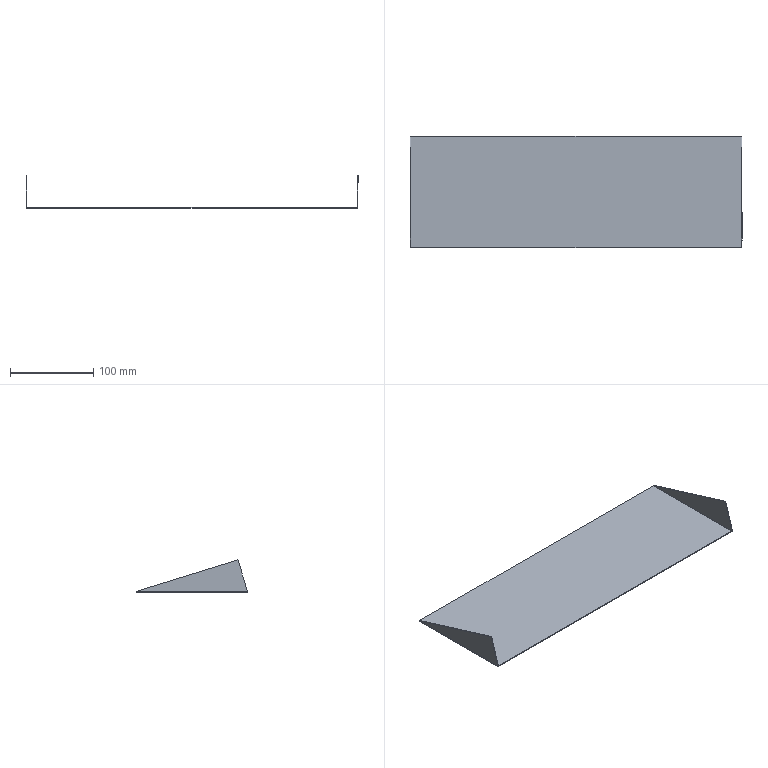Part | SolidWorks | features EdgeFlange 1, FlatPattern 1, MirrorPattern 1, SMBaseFlange 1, SheetMetal 1 | 1 solid | 20 faces | box 399.001 x 133.5 x 38.5 mm | volume 58192 mm3 | plane 12 | spline 4 | cylinder 4 | commonest cylinder face diameters 0.4 x2 2.4 x2
STEP:
#1=CARTESIAN_POINT('',(198.3,66.75,-1.));
#2=VERTEX_POINT('',#1);
#3=CARTESIAN_POINT('',(198.3,-66.75,-1.));
#4=VERTEX_POINT('',#3);
#5=CARTESIAN_POINT('',(198.3,66.75,-1.));
#6=DIRECTION('',(0.,-1.,0.));
#7=VECTOR('',#6,1000.);
#8=LINE('',#5,#7);
#9=EDGE_CURVE('',#2,#4,#8,.T.);
#10=ORIENTED_EDGE('',*,*,#9,.T.);
#11=CARTESIAN_POINT('',(-198.3,-66.75,-1.));
#12=VERTEX_POINT('',#11);
#13=CARTESIAN_POINT('',(-199.5,-66.75,-1.));
#14=DIRECTION('',(1.,0.,0.));
#15=VECTOR('',#14,1000.);
#16=LINE('',#13,#15);
#17=EDGE_CURVE('',#12,#4,#16,.T.);
#18=ORIENTED_EDGE('',*,*,#17,.F.);
#19=CARTESIAN_POINT('',(-198.3,66.75,-1.));
#20=VERTEX_POINT('',#19);
#21=CARTESIAN_POINT('',(-198.3,-66.75,-1.));
#22=DIRECTION('',(0.,1.,0.));
#23=VECTOR('',#22,1000.);
#24=LINE('',#21,#23);
#25=EDGE_CURVE('',#12,#20,#24,.T.);
#26=ORIENTED_EDGE('',*,*,#25,.T.);
#27=CARTESIAN_POINT('',(-199.5,66.75,-1.));
#28=DIRECTION('',(-1.,0.,0.));
#29=VECTOR('',#28,1000.);
#30=LINE('',#27,#29);
#31=EDGE_CURVE('',#2,#20,#30,.T.);
#32=ORIENTED_EDGE('',*,*,#31,.F.);
#33=EDGE_LOOP('',(#10,#18,#26,#32));
#34=FACE_OUTER_BOUND('',#33,.T.);
#35=CARTESIAN_POINT('',(0.,0.,-1.));
#36=DIRECTION('',(0.,0.,1.));
#37=DIRECTION('',(1.,0.,0.));
#38=AXIS2_PLACEMENT_3D('',#35,#36,#37);
#39=PLANE('',#38);
#40=ADVANCED_FACE('',(#34),#39,.F.);
#41=CARTESIAN_POINT('',(-198.3,-66.75,0.));
#42=VERTEX_POINT('',#41);
#43=CARTESIAN_POINT('',(198.3,-66.75,0.));
#44=VERTEX_POINT('',#43);
#45=CARTESIAN_POINT('',(-199.5,-66.75,0.));
#46=DIRECTION('',(1.,0.,0.));
#47=VECTOR('',#46,1000.);
#48=LINE('',#45,#47);
#49=EDGE_CURVE('',#42,#44,#48,.T.);
#50=ORIENTED_EDGE('',*,*,#49,.T.);
#51=CARTESIAN_POINT('',(198.3,66.75,0.));
#52=VERTEX_POINT('',#51);
#53=CARTESIAN_POINT('',(198.3,66.75,0.));
#54=DIRECTION('',(0.,-1.,0.));
#55=VECTOR('',#54,1000.);
#56=LINE('',#53,#55);
#57=EDGE_CURVE('',#52,#44,#56,.T.);
#58=ORIENTED_EDGE('',*,*,#57,.F.);
#59=CARTESIAN_POINT('',(-198.3,66.75,0.));
#60=VERTEX_POINT('',#59);
#61=CARTESIAN_POINT('',(-199.5,66.75,0.));
#62=DIRECTION('',(-1.,0.,0.));
#63=VECTOR('',#62,1000.);
#64=LINE('',#61,#63);
#65=EDGE_CURVE('',#52,#60,#64,.T.);
#66=ORIENTED_EDGE('',*,*,#65,.T.);
#67=CARTESIAN_POINT('',(-198.3,-66.75,0.));
#68=DIRECTION('',(0.,1.,0.));
#69=VECTOR('',#68,1000.);
#70=LINE('',#67,#69);
#71=EDGE_CURVE('',#42,#60,#70,.T.);
#72=ORIENTED_EDGE('',*,*,#71,.F.);
#73=EDGE_LOOP('',(#50,#58,#66,#72));
#74=FACE_OUTER_BOUND('',#73,.T.);
#75=CARTESIAN_POINT('',(0.,0.,0.));
#76=DIRECTION('',(0.,0.,1.));
#77=DIRECTION('',(1.,0.,0.));
#78=AXIS2_PLACEMENT_3D('',#75,#76,#77);
#79=PLANE('',#78);
#80=ADVANCED_FACE('',(#74),#79,.T.);
#81=ORIENTED_EDGE('',*,*,#65,.F.);
#82=CARTESIAN_POINT('',(198.3,66.75,0.));
#83=DIRECTION('',(0.,0.,-1.));
#84=VECTOR('',#83,1000.);
#85=LINE('',#82,#84);
#86=EDGE_CURVE('',#52,#2,#85,.T.);
#87=ORIENTED_EDGE('',*,*,#86,.T.);
#88=ORIENTED_EDGE('',*,*,#31,.T.);
#89=CARTESIAN_POINT('',(-198.3,66.75,0.));
#90=DIRECTION('',(0.,0.,-1.));
#91=VECTOR('',#90,1000.);
#92=LINE('',#89,#91);
#93=EDGE_CURVE('',#60,#20,#92,.T.);
#94=ORIENTED_EDGE('',*,*,#93,.F.);
#95=EDGE_LOOP('',(#81,#87,#88,#94));
#96=FACE_OUTER_BOUND('',#95,.T.);
#97=CARTESIAN_POINT('',(-199.5,66.75,-1.));
#98=DIRECTION('',(0.,1.,0.));
#99=DIRECTION('',(0.,0.,1.));
#100=AXIS2_PLACEMENT_3D('',#97,#98,#99);
#101=PLANE('',#100);
#102=ADVANCED_FACE('',(#96),#101,.T.);
#103=CARTESIAN_POINT('',(198.3,-66.75,0.));
#104=DIRECTION('',(0.,0.,-1.));
#105=VECTOR('',#104,1000.);
#106=LINE('',#103,#105);
#107=EDGE_CURVE('',#44,#4,#106,.T.);
#108=ORIENTED_EDGE('',*,*,#107,.F.);
#109=ORIENTED_EDGE('',*,*,#49,.F.);
#110=CARTESIAN_POINT('',(-198.3,-66.75,0.));
#111=DIRECTION('',(0.,0.,-1.));
#112=VECTOR('',#111,1000.);
#113=LINE('',#110,#112);
#114=EDGE_CURVE('',#42,#12,#113,.T.);
#115=ORIENTED_EDGE('',*,*,#114,.T.);
#116=ORIENTED_EDGE('',*,*,#17,.T.);
#117=EDGE_LOOP('',(#108,#109,#115,#116));
#118=FACE_OUTER_BOUND('',#117,.T.);
#119=CARTESIAN_POINT('',(-199.5,-66.75,-1.));
#120=DIRECTION('',(0.,-1.,0.));
#121=DIRECTION('',(0.,0.,-1.));
#122=AXIS2_PLACEMENT_3D('',#119,#120,#121);
#123=PLANE('',#122);
#124=ADVANCED_FACE('',(#118),#123,.T.);
#125=CARTESIAN_POINT('',(-198.5,66.099,0.2));
#126=VERTEX_POINT('',#125);
#127=CARTESIAN_POINT('',(-199.5,66.099,0.2));
#128=VERTEX_POINT('',#127);
#129=CARTESIAN_POINT('',(-199.5,66.099,0.2));
#130=DIRECTION('',(-1.,0.,0.));
#131=VECTOR('',#130,1000.);
#132=LINE('',#129,#131);
#133=EDGE_CURVE('',#126,#128,#132,.T.);
#134=ORIENTED_EDGE('',*,*,#133,.F.);
#135=CARTESIAN_POINT('',(-198.3,66.75,0.));
#136=CARTESIAN_POINT('',(-198.352,66.642,0.));
#137=CARTESIAN_POINT('',(-198.404,66.533,0.02155));
#138=CARTESIAN_POINT('',(-198.478,66.316,0.0956));
#139=CARTESIAN_POINT('',(-198.5,66.208,0.1476));
#140=CARTESIAN_POINT('',(-198.5,66.099,0.2));
#141=B_SPLINE_CURVE_WITH_KNOTS('',3,(#135,#136,#137,#138,#139,#140),.UNSPECIFIED.,.F.,.F.,(4,2,4),(0.,0.5,1.),.UNSPECIFIED.);
#142=EDGE_CURVE('',#60,#126,#141,.T.);
#143=ORIENTED_EDGE('',*,*,#142,.F.);
#144=ORIENTED_EDGE('',*,*,#93,.T.);
#145=CARTESIAN_POINT('',(-198.3,66.75,-1.));
#146=CARTESIAN_POINT('',(-198.459,66.695,-1.));
#147=CARTESIAN_POINT('',(-198.612,66.642,-0.9696));
#148=CARTESIAN_POINT('',(-198.904,66.533,-0.8489));
#149=CARTESIAN_POINT('',(-199.036,66.48,-0.761));
#150=CARTESIAN_POINT('',(-199.26,66.371,-0.5375));
#151=CARTESIAN_POINT('',(-199.348,66.317,-0.4053));
#152=CARTESIAN_POINT('',(-199.469,66.208,-0.1145));
#153=CARTESIAN_POINT('',(-199.5,66.154,0.04138));
#154=CARTESIAN_POINT('',(-199.5,66.099,0.2));
#155=B_SPLINE_CURVE_WITH_KNOTS('',3,(#145,#146,#147,#148,#149,#150,#151,#152,#153,#154),.UNSPECIFIED.,.F.,.F.,(4,2,2,2,4),(0.,0.0004941,0.0009882,0.001482,0.001976),.UNSPECIFIED.);
#156=EDGE_CURVE('',#20,#128,#155,.T.);
#157=ORIENTED_EDGE('',*,*,#156,.T.);
#158=EDGE_LOOP('',(#134,#143,#144,#157));
#159=FACE_OUTER_BOUND('',#158,.T.);
#160=CARTESIAN_POINT('',(-198.3,66.75,-1.01));
#161=CARTESIAN_POINT('',(-198.458,66.696,-1.01));
#162=CARTESIAN_POINT('',(-198.617,66.642,-0.9785));
#163=CARTESIAN_POINT('',(-198.909,66.533,-0.8573));
#164=CARTESIAN_POINT('',(-199.044,66.479,-0.7676));
#165=CARTESIAN_POINT('',(-199.268,66.371,-0.5436));
#166=CARTESIAN_POINT('',(-199.357,66.316,-0.4094));
#167=CARTESIAN_POINT('',(-199.479,66.208,-0.1167));
#168=CARTESIAN_POINT('',(-199.51,66.154,0.04159));
#169=CARTESIAN_POINT('',(-199.51,66.099,0.2));
#170=CARTESIAN_POINT('',(-198.3,66.75,-1.));
#171=CARTESIAN_POINT('',(-198.457,66.696,-1.));
#172=CARTESIAN_POINT('',(-198.614,66.642,-0.9688));
#173=CARTESIAN_POINT('',(-198.904,66.533,-0.8485));
#174=CARTESIAN_POINT('',(-199.037,66.479,-0.7596));
#175=CARTESIAN_POINT('',(-199.26,66.371,-0.5375));
#176=CARTESIAN_POINT('',(-199.349,66.316,-0.4043));
#177=CARTESIAN_POINT('',(-199.469,66.208,-0.1141));
#178=CARTESIAN_POINT('',(-199.5,66.154,0.0429));
#179=CARTESIAN_POINT('',(-199.5,66.099,0.2));
#180=CARTESIAN_POINT('',(-198.3,66.75,0.));
#181=CARTESIAN_POINT('',(-198.326,66.696,0.));
#182=CARTESIAN_POINT('',(-198.352,66.642,0.005205));
#183=CARTESIAN_POINT('',(-198.401,66.533,0.02524));
#184=CARTESIAN_POINT('',(-198.423,66.479,0.04007));
#185=CARTESIAN_POINT('',(-198.46,66.371,0.07709));
#186=CARTESIAN_POINT('',(-198.475,66.316,0.09928));
#187=CARTESIAN_POINT('',(-198.495,66.208,0.1477));
#188=CARTESIAN_POINT('',(-198.5,66.154,0.1738));
#189=CARTESIAN_POINT('',(-198.5,66.099,0.2));
#190=B_SPLINE_SURFACE_WITH_KNOTS('',1,3,((#160,#161,#162,#163,#164,#165,#166,#167,#168,#169),(#170,#171,#172,#173,#174,#175,#176,#177,#178,#179),(#180,#181,#182,#183,#184,#185,#186,#187,#188,#189)),.UNSPECIFIED.,.F.,.F.,.F.,(2,1,2),(4,2,2,2,4),(-0.01,0.,1.),(0.,0.25,0.5,0.75,1.),.UNSPECIFIED.);
#191=ADVANCED_FACE('',(#159),#190,.F.);
#192=CARTESIAN_POINT('',(-198.5,-66.689,0.2));
#193=VERTEX_POINT('',#192);
#194=CARTESIAN_POINT('',(-198.5,-66.689,0.2));
#195=CARTESIAN_POINT('',(-198.5,-66.699,0.1476));
#196=CARTESIAN_POINT('',(-198.478,-66.709,0.0956));
#197=CARTESIAN_POINT('',(-198.404,-66.73,0.02155));
#198=CARTESIAN_POINT('',(-198.352,-66.74,0.));
#199=CARTESIAN_POINT('',(-198.3,-66.75,0.));
#200=B_SPLINE_CURVE_WITH_KNOTS('',3,(#194,#195,#196,#197,#198,#199),.UNSPECIFIED.,.F.,.F.,(4,2,4),(0.,0.5,1.),.UNSPECIFIED.);
#201=EDGE_CURVE('',#193,#42,#200,.T.);
#202=ORIENTED_EDGE('',*,*,#201,.F.);
#203=CARTESIAN_POINT('',(-199.5,-66.689,0.2));
#204=VERTEX_POINT('',#203);
#205=CARTESIAN_POINT('',(-198.5,-66.689,0.2));
#206=DIRECTION('',(-1.,0.,0.));
#207=VECTOR('',#206,1000.);
#208=LINE('',#205,#207);
#209=EDGE_CURVE('',#193,#204,#208,.T.);
#210=ORIENTED_EDGE('',*,*,#209,.T.);
#211=CARTESIAN_POINT('',(-199.5,-66.689,0.2));
#212=CARTESIAN_POINT('',(-199.5,-66.694,0.04292));
#213=CARTESIAN_POINT('',(-199.469,-66.699,-0.1141));
#214=CARTESIAN_POINT('',(-199.349,-66.709,-0.4043));
#215=CARTESIAN_POINT('',(-199.26,-66.714,-0.5375));
#216=CARTESIAN_POINT('',(-199.037,-66.724,-0.7596));
#217=CARTESIAN_POINT('',(-198.904,-66.73,-0.8485));
#218=CARTESIAN_POINT('',(-198.614,-66.74,-0.9688));
#219=CARTESIAN_POINT('',(-198.457,-66.745,-1.));
#220=CARTESIAN_POINT('',(-198.3,-66.75,-1.));
#221=B_SPLINE_CURVE_WITH_KNOTS('',3,(#211,#212,#213,#214,#215,#216,#217,#218,#219,#220),.UNSPECIFIED.,.F.,.F.,(4,2,2,2,4),(0.,0.25,0.5,0.75,1.),.UNSPECIFIED.);
#222=EDGE_CURVE('',#204,#12,#221,.T.);
#223=ORIENTED_EDGE('',*,*,#222,.T.);
#224=ORIENTED_EDGE('',*,*,#114,.F.);
#225=EDGE_LOOP('',(#202,#210,#223,#224));
#226=FACE_OUTER_BOUND('',#225,.T.);
#227=CARTESIAN_POINT('',(-199.51,-66.689,0.2));
#228=CARTESIAN_POINT('',(-199.51,-66.694,0.04158));
#229=CARTESIAN_POINT('',(-199.479,-66.699,-0.1167));
#230=CARTESIAN_POINT('',(-199.357,-66.709,-0.4094));
#231=CARTESIAN_POINT('',(-199.268,-66.714,-0.5436));
#232=CARTESIAN_POINT('',(-199.044,-66.724,-0.7676));
#233=CARTESIAN_POINT('',(-198.909,-66.73,-0.8573));
#234=CARTESIAN_POINT('',(-198.617,-66.74,-0.9785));
#235=CARTESIAN_POINT('',(-198.458,-66.745,-1.01));
#236=CARTESIAN_POINT('',(-198.3,-66.75,-1.01));
#237=CARTESIAN_POINT('',(-199.5,-66.689,0.2));
#238=CARTESIAN_POINT('',(-199.5,-66.694,0.04289));
#239=CARTESIAN_POINT('',(-199.469,-66.699,-0.1141));
#240=CARTESIAN_POINT('',(-199.349,-66.709,-0.4043));
#241=CARTESIAN_POINT('',(-199.26,-66.714,-0.5375));
#242=CARTESIAN_POINT('',(-199.037,-66.724,-0.7596));
#243=CARTESIAN_POINT('',(-198.904,-66.73,-0.8485));
#244=CARTESIAN_POINT('',(-198.614,-66.74,-0.9688));
#245=CARTESIAN_POINT('',(-198.457,-66.745,-1.));
#246=CARTESIAN_POINT('',(-198.3,-66.75,-1.));
#247=CARTESIAN_POINT('',(-198.5,-66.689,0.2));
#248=CARTESIAN_POINT('',(-198.5,-66.694,0.1738));
#249=CARTESIAN_POINT('',(-198.495,-66.699,0.1477));
#250=CARTESIAN_POINT('',(-198.475,-66.709,0.09928));
#251=CARTESIAN_POINT('',(-198.46,-66.714,0.07709));
#252=CARTESIAN_POINT('',(-198.423,-66.724,0.04007));
#253=CARTESIAN_POINT('',(-198.401,-66.73,0.02524));
#254=CARTESIAN_POINT('',(-198.352,-66.74,0.005205));
#255=CARTESIAN_POINT('',(-198.326,-66.745,0.));
#256=CARTESIAN_POINT('',(-198.3,-66.75,0.));
#257=CARTESIAN_POINT('',(-198.49,-66.689,0.2));
#258=CARTESIAN_POINT('',(-198.49,-66.694,0.1751));
#259=CARTESIAN_POINT('',(-198.485,-66.699,0.1503));
#260=CARTESIAN_POINT('',(-198.466,-66.709,0.1044));
#261=CARTESIAN_POINT('',(-198.452,-66.714,0.0833));
#262=CARTESIAN_POINT('',(-198.417,-66.724,0.04814));
#263=CARTESIAN_POINT('',(-198.396,-66.73,0.03407));
#264=CARTESIAN_POINT('',(-198.35,-66.74,0.01504));
#265=CARTESIAN_POINT('',(-198.325,-66.745,0.0101));
#266=CARTESIAN_POINT('',(-198.3,-66.75,0.0101));
#267=B_SPLINE_SURFACE_WITH_KNOTS('',1,3,((#227,#228,#229,#230,#231,#232,#233,#234,#235,#236),(#237,#238,#239,#240,#241,#242,#243,#244,#245,#246),(#247,#248,#249,#250,#251,#252,#253,#254,#255,#256),(#257,#258,#259,#260,#261,#262,#263,#264,#265,#266)),.UNSPECIFIED.,.F.,.F.,.F.,(2,1,1,2),(4,2,2,2,4),(-0.01,0.,1.,1.01),(0.,0.25,0.5,0.75,1.),.UNSPECIFIED.);
#268=ADVANCED_FACE('',(#226),#267,.F.);
#269=ORIENTED_EDGE('',*,*,#25,.F.);
#270=ORIENTED_EDGE('',*,*,#222,.F.);
#271=CARTESIAN_POINT('',(-199.5,66.099,0.2));
#272=DIRECTION('',(0.,1.,0.));
#273=VECTOR('',#272,1000.);
#274=LINE('',#271,#273);
#275=EDGE_CURVE('',#204,#128,#274,.T.);
#276=ORIENTED_EDGE('',*,*,#275,.T.);
#277=ORIENTED_EDGE('',*,*,#156,.F.);
#278=EDGE_LOOP('',(#269,#270,#276,#277));
#279=FACE_OUTER_BOUND('',#278,.T.);
#280=CARTESIAN_POINT('',(-198.3,-66.75,0.2));
#281=DIRECTION('',(0.,-1.,0.));
#282=DIRECTION('',(-1.,0.,0.));
#283=AXIS2_PLACEMENT_3D('',#280,#281,#282);
#284=CYLINDRICAL_SURFACE('',#283,1.2);
#285=ADVANCED_FACE('',(#279),#284,.T.);
#286=ORIENTED_EDGE('',*,*,#71,.T.);
#287=ORIENTED_EDGE('',*,*,#142,.T.);
#288=CARTESIAN_POINT('',(-198.5,66.099,0.2));
#289=DIRECTION('',(0.,-1.,0.));
#290=VECTOR('',#289,1000.);
#291=LINE('',#288,#290);
#292=EDGE_CURVE('',#126,#193,#291,.T.);
#293=ORIENTED_EDGE('',*,*,#292,.T.);
#294=ORIENTED_EDGE('',*,*,#201,.T.);
#295=EDGE_LOOP('',(#286,#287,#293,#294));
#296=FACE_OUTER_BOUND('',#295,.T.);
#297=CARTESIAN_POINT('',(-198.3,-66.75,0.2));
#298=DIRECTION('',(0.,-1.,0.));
#299=DIRECTION('',(-1.,0.,0.));
#300=AXIS2_PLACEMENT_3D('',#297,#298,#299);
#301=CYLINDRICAL_SURFACE('',#300,0.2);
#302=ADVANCED_FACE('',(#296),#301,.F.);
#303=ORIENTED_EDGE('',*,*,#133,.T.);
#304=CARTESIAN_POINT('',(-199.5,-55.221,37.5));
#305=VERTEX_POINT('',#304);
#306=CARTESIAN_POINT('',(-199.5,5.765,18.75));
#307=DIRECTION('',(0.,0.9558,-0.2939));
#308=VECTOR('',#307,1000.);
#309=LINE('',#306,#308);
#310=EDGE_CURVE('',#305,#128,#309,.T.);
#311=ORIENTED_EDGE('',*,*,#310,.F.);
#312=CARTESIAN_POINT('',(-198.5,-55.221,37.5));
#313=VERTEX_POINT('',#312);
#314=CARTESIAN_POINT('',(-199.5,-55.221,37.5));
#315=DIRECTION('',(1.,0.,0.));
#316=VECTOR('',#315,1000.);
#317=LINE('',#314,#316);
#318=EDGE_CURVE('',#305,#313,#317,.T.);
#319=ORIENTED_EDGE('',*,*,#318,.T.);
#320=CARTESIAN_POINT('',(-198.5,-55.221,37.5));
#321=DIRECTION('',(0.,0.9558,-0.2939));
#322=VECTOR('',#321,1000.);
#323=LINE('',#320,#322);
#324=EDGE_CURVE('',#313,#126,#323,.T.);
#325=ORIENTED_EDGE('',*,*,#324,.T.);
#326=EDGE_LOOP('',(#303,#311,#319,#325));
#327=FACE_OUTER_BOUND('',#326,.T.);
#328=CARTESIAN_POINT('',(-199.5,-55.221,37.5));
#329=DIRECTION('',(0.,-0.2939,-0.9558));
#330=DIRECTION('',(0.,0.9558,-0.2939));
#331=AXIS2_PLACEMENT_3D('',#328,#329,#330);
#332=PLANE('',#331);
#333=ADVANCED_FACE('',(#327),#332,.F.);
#334=ORIENTED_EDGE('',*,*,#209,.F.);
#335=CARTESIAN_POINT('',(-198.5,-66.75,0.));
#336=DIRECTION('',(0.,0.2939,0.9558));
#337=VECTOR('',#336,1000.);
#338=LINE('',#335,#337);
#339=EDGE_CURVE('',#193,#313,#338,.T.);
#340=ORIENTED_EDGE('',*,*,#339,.T.);
#341=ORIENTED_EDGE('',*,*,#318,.F.);
#342=CARTESIAN_POINT('',(-199.5,-60.985,18.75));
#343=DIRECTION('',(0.,0.2939,0.9558));
#344=VECTOR('',#343,1000.);
#345=LINE('',#342,#344);
#346=EDGE_CURVE('',#204,#305,#345,.T.);
#347=ORIENTED_EDGE('',*,*,#346,.F.);
#348=EDGE_LOOP('',(#334,#340,#341,#347));
#349=FACE_OUTER_BOUND('',#348,.T.);
#350=CARTESIAN_POINT('',(-199.5,-66.75,0.));
#351=DIRECTION('',(0.,0.9558,-0.2939));
#352=DIRECTION('',(0.,0.2939,0.9558));
#353=AXIS2_PLACEMENT_3D('',#350,#351,#352);
#354=PLANE('',#353);
#355=ADVANCED_FACE('',(#349),#354,.F.);
#356=ORIENTED_EDGE('',*,*,#275,.F.);
#357=ORIENTED_EDGE('',*,*,#346,.T.);
#358=ORIENTED_EDGE('',*,*,#310,.T.);
#359=EDGE_LOOP('',(#356,#357,#358));
#360=FACE_OUTER_BOUND('',#359,.T.);
#361=CARTESIAN_POINT('',(-199.5,0.,0.));
#362=DIRECTION('',(1.,0.,0.));
#363=DIRECTION('',(0.,0.,-1.));
#364=AXIS2_PLACEMENT_3D('',#361,#362,#363);
#365=PLANE('',#364);
#366=ADVANCED_FACE('',(#360),#365,.F.);
#367=ORIENTED_EDGE('',*,*,#339,.F.);
#368=ORIENTED_EDGE('',*,*,#292,.F.);
#369=ORIENTED_EDGE('',*,*,#324,.F.);
#370=EDGE_LOOP('',(#367,#368,#369));
#371=FACE_OUTER_BOUND('',#370,.T.);
#372=CARTESIAN_POINT('',(-198.5,0.,0.));
#373=DIRECTION('',(1.,0.,0.));
#374=DIRECTION('',(0.,0.,-1.));
#375=AXIS2_PLACEMENT_3D('',#372,#373,#374);
#376=PLANE('',#375);
#377=ADVANCED_FACE('',(#371),#376,.T.);
#378=CARTESIAN_POINT('',(198.5,-66.689,0.2));
#379=VERTEX_POINT('',#378);
#380=CARTESIAN_POINT('',(199.5,-66.689,0.2));
#381=VERTEX_POINT('',#380);
#382=CARTESIAN_POINT('',(199.5,-66.689,0.2));
#383=DIRECTION('',(1.,0.,0.));
#384=VECTOR('',#383,1000.);
#385=LINE('',#382,#384);
#386=EDGE_CURVE('',#379,#381,#385,.T.);
#387=ORIENTED_EDGE('',*,*,#386,.F.);
#388=CARTESIAN_POINT('',(198.3,-66.75,0.));
#389=CARTESIAN_POINT('',(198.352,-66.74,0.));
#390=CARTESIAN_POINT('',(198.404,-66.73,0.02155));
#391=CARTESIAN_POINT('',(198.478,-66.709,0.0956));
#392=CARTESIAN_POINT('',(198.5,-66.699,0.1476));
#393=CARTESIAN_POINT('',(198.5,-66.689,0.2));
#394=B_SPLINE_CURVE_WITH_KNOTS('',3,(#388,#389,#390,#391,#392,#393),.UNSPECIFIED.,.F.,.F.,(4,2,4),(0.,0.5,1.),.UNSPECIFIED.);
#395=EDGE_CURVE('',#44,#379,#394,.T.);
#396=ORIENTED_EDGE('',*,*,#395,.F.);
#397=ORIENTED_EDGE('',*,*,#107,.T.);
#398=CARTESIAN_POINT('',(198.3,-66.75,-1.));
#399=CARTESIAN_POINT('',(198.457,-66.745,-1.));
#400=CARTESIAN_POINT('',(198.614,-66.74,-0.9688));
#401=CARTESIAN_POINT('',(198.904,-66.73,-0.8485));
#402=CARTESIAN_POINT('',(199.037,-66.724,-0.7596));
#403=CARTESIAN_POINT('',(199.26,-66.714,-0.5375));
#404=CARTESIAN_POINT('',(199.349,-66.709,-0.4043));
#405=CARTESIAN_POINT('',(199.469,-66.699,-0.1141));
#406=CARTESIAN_POINT('',(199.5,-66.694,0.04292));
#407=CARTESIAN_POINT('',(199.5,-66.689,0.2));
#408=B_SPLINE_CURVE_WITH_KNOTS('',3,(#398,#399,#400,#401,#402,#403,#404,#405,#406,#407),.UNSPECIFIED.,.F.,.F.,(4,2,2,2,4),(0.,0.25,0.5,0.75,1.),.UNSPECIFIED.);
#409=EDGE_CURVE('',#4,#381,#408,.T.);
#410=ORIENTED_EDGE('',*,*,#409,.T.);
#411=EDGE_LOOP('',(#387,#396,#397,#410));
#412=FACE_OUTER_BOUND('',#411,.T.);
#413=CARTESIAN_POINT('',(198.3,-66.75,-1.01));
#414=CARTESIAN_POINT('',(198.458,-66.745,-1.01));
#415=CARTESIAN_POINT('',(198.617,-66.74,-0.9785));
#416=CARTESIAN_POINT('',(198.909,-66.73,-0.8573));
#417=CARTESIAN_POINT('',(199.044,-66.724,-0.7676));
#418=CARTESIAN_POINT('',(199.268,-66.714,-0.5436));
#419=CARTESIAN_POINT('',(199.357,-66.709,-0.4094));
#420=CARTESIAN_POINT('',(199.479,-66.699,-0.1167));
#421=CARTESIAN_POINT('',(199.51,-66.694,0.04158));
#422=CARTESIAN_POINT('',(199.51,-66.689,0.2));
#423=CARTESIAN_POINT('',(198.3,-66.75,-1.));
#424=CARTESIAN_POINT('',(198.457,-66.745,-1.));
#425=CARTESIAN_POINT('',(198.614,-66.74,-0.9688));
#426=CARTESIAN_POINT('',(198.904,-66.73,-0.8485));
#427=CARTESIAN_POINT('',(199.037,-66.724,-0.7596));
#428=CARTESIAN_POINT('',(199.26,-66.714,-0.5375));
#429=CARTESIAN_POINT('',(199.349,-66.709,-0.4043));
#430=CARTESIAN_POINT('',(199.469,-66.699,-0.1141));
#431=CARTESIAN_POINT('',(199.5,-66.694,0.04289));
#432=CARTESIAN_POINT('',(199.5,-66.689,0.2));
#433=CARTESIAN_POINT('',(198.3,-66.75,0.));
#434=CARTESIAN_POINT('',(198.326,-66.745,0.));
#435=CARTESIAN_POINT('',(198.352,-66.74,0.005205));
#436=CARTESIAN_POINT('',(198.401,-66.73,0.02524));
#437=CARTESIAN_POINT('',(198.423,-66.724,0.04007));
#438=CARTESIAN_POINT('',(198.46,-66.714,0.07709));
#439=CARTESIAN_POINT('',(198.475,-66.709,0.09928));
#440=CARTESIAN_POINT('',(198.495,-66.699,0.1477));
#441=CARTESIAN_POINT('',(198.5,-66.694,0.1738));
#442=CARTESIAN_POINT('',(198.5,-66.689,0.2));
#443=CARTESIAN_POINT('',(198.3,-66.75,0.0101));
#444=CARTESIAN_POINT('',(198.325,-66.745,0.0101));
#445=CARTESIAN_POINT('',(198.35,-66.74,0.01504));
#446=CARTESIAN_POINT('',(198.396,-66.73,0.03407));
#447=CARTESIAN_POINT('',(198.417,-66.724,0.04814));
#448=CARTESIAN_POINT('',(198.452,-66.714,0.0833));
#449=CARTESIAN_POINT('',(198.466,-66.709,0.1044));
#450=CARTESIAN_POINT('',(198.485,-66.699,0.1503));
#451=CARTESIAN_POINT('',(198.49,-66.694,0.1751));
#452=CARTESIAN_POINT('',(198.49,-66.689,0.2));
#453=B_SPLINE_SURFACE_WITH_KNOTS('',1,3,((#413,#414,#415,#416,#417,#418,#419,#420,#421,#422),(#423,#424,#425,#426,#427,#428,#429,#430,#431,#432),(#433,#434,#435,#436,#437,#438,#439,#440,#441,#442),(#443,#444,#445,#446,#447,#448,#449,#450,#451,#452)),.UNSPECIFIED.,.F.,.F.,.F.,(2,1,1,2),(4,2,2,2,4),(-0.01,0.,1.,1.01),(0.,0.25,0.5,0.75,1.),.UNSPECIFIED.);
#454=ADVANCED_FACE('',(#412),#453,.F.);
#455=CARTESIAN_POINT('',(198.5,66.099,0.2));
#456=VERTEX_POINT('',#455);
#457=CARTESIAN_POINT('',(198.5,66.099,0.2));
#458=CARTESIAN_POINT('',(198.5,66.208,0.1476));
#459=CARTESIAN_POINT('',(198.478,66.316,0.0956));
#460=CARTESIAN_POINT('',(198.404,66.533,0.02155));
#461=CARTESIAN_POINT('',(198.352,66.642,0.));
#462=CARTESIAN_POINT('',(198.3,66.75,0.));
#463=B_SPLINE_CURVE_WITH_KNOTS('',3,(#457,#458,#459,#460,#461,#462),.UNSPECIFIED.,.F.,.F.,(4,2,4),(0.,0.5,1.),.UNSPECIFIED.);
#464=EDGE_CURVE('',#456,#52,#463,.T.);
#465=ORIENTED_EDGE('',*,*,#464,.F.);
#466=CARTESIAN_POINT('',(199.5,66.099,0.2));
#467=VERTEX_POINT('',#466);
#468=CARTESIAN_POINT('',(198.5,66.099,0.2));
#469=DIRECTION('',(1.,0.,0.));
#470=VECTOR('',#469,1000.);
#471=LINE('',#468,#470);
#472=EDGE_CURVE('',#456,#467,#471,.T.);
#473=ORIENTED_EDGE('',*,*,#472,.T.);
#474=CARTESIAN_POINT('',(199.5,66.099,0.2));
#475=CARTESIAN_POINT('',(199.5,66.154,0.04138));
#476=CARTESIAN_POINT('',(199.47,66.207,-0.1117));
#477=CARTESIAN_POINT('',(199.349,66.316,-0.4041));
#478=CARTESIAN_POINT('',(199.261,66.37,-0.5359));
#479=CARTESIAN_POINT('',(199.038,66.479,-0.7597));
#480=CARTESIAN_POINT('',(198.905,66.533,-0.848));
#481=CARTESIAN_POINT('',(198.614,66.641,-0.9687));
#482=CARTESIAN_POINT('',(198.459,66.695,-1.));
#483=CARTESIAN_POINT('',(198.3,66.75,-1.));
#484=B_SPLINE_CURVE_WITH_KNOTS('',3,(#474,#475,#476,#477,#478,#479,#480,#481,#482,#483),.UNSPECIFIED.,.F.,.F.,(4,2,2,2,4),(0.,0.0004941,0.0009882,0.001482,0.001976),.UNSPECIFIED.);
#485=EDGE_CURVE('',#467,#2,#484,.T.);
#486=ORIENTED_EDGE('',*,*,#485,.T.);
#487=ORIENTED_EDGE('',*,*,#86,.F.);
#488=EDGE_LOOP('',(#465,#473,#486,#487));
#489=FACE_OUTER_BOUND('',#488,.T.);
#490=CARTESIAN_POINT('',(199.51,66.099,0.2));
#491=CARTESIAN_POINT('',(199.51,66.154,0.04159));
#492=CARTESIAN_POINT('',(199.479,66.208,-0.1167));
#493=CARTESIAN_POINT('',(199.357,66.316,-0.4094));
#494=CARTESIAN_POINT('',(199.268,66.371,-0.5436));
#495=CARTESIAN_POINT('',(199.044,66.479,-0.7676));
#496=CARTESIAN_POINT('',(198.909,66.533,-0.8573));
#497=CARTESIAN_POINT('',(198.617,66.642,-0.9785));
#498=CARTESIAN_POINT('',(198.458,66.696,-1.01));
#499=CARTESIAN_POINT('',(198.3,66.75,-1.01));
#500=CARTESIAN_POINT('',(199.5,66.099,0.2));
#501=CARTESIAN_POINT('',(199.5,66.154,0.0429));
#502=CARTESIAN_POINT('',(199.469,66.208,-0.1141));
#503=CARTESIAN_POINT('',(199.349,66.316,-0.4043));
#504=CARTESIAN_POINT('',(199.26,66.371,-0.5375));
#505=CARTESIAN_POINT('',(199.037,66.479,-0.7596));
#506=CARTESIAN_POINT('',(198.904,66.533,-0.8485));
#507=CARTESIAN_POINT('',(198.614,66.642,-0.9688));
#508=CARTESIAN_POINT('',(198.457,66.696,-1.));
#509=CARTESIAN_POINT('',(198.3,66.75,-1.));
#510=CARTESIAN_POINT('',(198.5,66.099,0.2));
#511=CARTESIAN_POINT('',(198.5,66.154,0.1738));
#512=CARTESIAN_POINT('',(198.495,66.208,0.1477));
#513=CARTESIAN_POINT('',(198.475,66.316,0.09928));
#514=CARTESIAN_POINT('',(198.46,66.371,0.07709));
#515=CARTESIAN_POINT('',(198.423,66.479,0.04007));
#516=CARTESIAN_POINT('',(198.401,66.533,0.02524));
#517=CARTESIAN_POINT('',(198.352,66.642,0.005205));
#518=CARTESIAN_POINT('',(198.326,66.696,0.));
#519=CARTESIAN_POINT('',(198.3,66.75,0.));
#520=B_SPLINE_SURFACE_WITH_KNOTS('',1,3,((#490,#491,#492,#493,#494,#495,#496,#497,#498,#499),(#500,#501,#502,#503,#504,#505,#506,#507,#508,#509),(#510,#511,#512,#513,#514,#515,#516,#517,#518,#519)),.UNSPECIFIED.,.F.,.F.,.F.,(2,1,2),(4,2,2,2,4),(-0.01,0.,1.),(0.,0.25,0.5,0.75,1.),.UNSPECIFIED.);
#521=ADVANCED_FACE('',(#489),#520,.F.);
#522=ORIENTED_EDGE('',*,*,#9,.F.);
#523=ORIENTED_EDGE('',*,*,#485,.F.);
#524=CARTESIAN_POINT('',(199.5,-66.689,0.2));
#525=DIRECTION('',(0.,-1.,0.));
#526=VECTOR('',#525,1000.);
#527=LINE('',#524,#526);
#528=EDGE_CURVE('',#467,#381,#527,.T.);
#529=ORIENTED_EDGE('',*,*,#528,.T.);
#530=ORIENTED_EDGE('',*,*,#409,.F.);
#531=EDGE_LOOP('',(#522,#523,#529,#530));
#532=FACE_OUTER_BOUND('',#531,.T.);
#533=CARTESIAN_POINT('',(198.3,66.75,0.2));
#534=DIRECTION('',(0.,1.,0.));
#535=DIRECTION('',(1.,0.,0.));
#536=AXIS2_PLACEMENT_3D('',#533,#534,#535);
#537=CYLINDRICAL_SURFACE('',#536,1.2);
#538=ADVANCED_FACE('',(#532),#537,.T.);
#539=ORIENTED_EDGE('',*,*,#57,.T.);
#540=ORIENTED_EDGE('',*,*,#395,.T.);
#541=CARTESIAN_POINT('',(198.5,-66.689,0.2));
#542=DIRECTION('',(0.,1.,0.));
#543=VECTOR('',#542,1000.);
#544=LINE('',#541,#543);
#545=EDGE_CURVE('',#379,#456,#544,.T.);
#546=ORIENTED_EDGE('',*,*,#545,.T.);
#547=ORIENTED_EDGE('',*,*,#464,.T.);
#548=EDGE_LOOP('',(#539,#540,#546,#547));
#549=FACE_OUTER_BOUND('',#548,.T.);
#550=CARTESIAN_POINT('',(198.3,66.75,0.2));
#551=DIRECTION('',(0.,1.,0.));
#552=DIRECTION('',(1.,0.,0.));
#553=AXIS2_PLACEMENT_3D('',#550,#551,#552);
#554=CYLINDRICAL_SURFACE('',#553,0.2);
#555=ADVANCED_FACE('',(#549),#554,.F.);
#556=CARTESIAN_POINT('',(199.5,-55.221,37.5));
#557=VERTEX_POINT('',#556);
#558=CARTESIAN_POINT('',(199.5,-55.221,37.5));
#559=DIRECTION('',(0.,0.9558,-0.2939));
#560=VECTOR('',#559,1000.);
#561=LINE('',#558,#560);
#562=EDGE_CURVE('',#557,#467,#561,.T.);
#563=ORIENTED_EDGE('',*,*,#562,.T.);
#564=ORIENTED_EDGE('',*,*,#472,.F.);
#565=CARTESIAN_POINT('',(198.5,-55.221,37.5));
#566=VERTEX_POINT('',#565);
#567=CARTESIAN_POINT('',(198.5,5.765,18.75));
#568=DIRECTION('',(0.,0.9558,-0.2939));
#569=VECTOR('',#568,1000.);
#570=LINE('',#567,#569);
#571=EDGE_CURVE('',#566,#456,#570,.T.);
#572=ORIENTED_EDGE('',*,*,#571,.F.);
#573=CARTESIAN_POINT('',(199.5,-55.221,37.5));
#574=DIRECTION('',(-1.,0.,0.));
#575=VECTOR('',#574,1000.);
#576=LINE('',#573,#575);
#577=EDGE_CURVE('',#557,#566,#576,.T.);
#578=ORIENTED_EDGE('',*,*,#577,.F.);
#579=EDGE_LOOP('',(#563,#564,#572,#578));
#580=FACE_OUTER_BOUND('',#579,.T.);
#581=CARTESIAN_POINT('',(199.5,-55.221,37.5));
#582=DIRECTION('',(0.,0.2939,0.9558));
#583=DIRECTION('',(0.,-0.9558,0.2939));
#584=AXIS2_PLACEMENT_3D('',#581,#582,#583);
#585=PLANE('',#584);
#586=ADVANCED_FACE('',(#580),#585,.T.);
#587=CARTESIAN_POINT('',(198.5,-60.985,18.75));
#588=DIRECTION('',(0.,0.2939,0.9558));
#589=VECTOR('',#588,1000.);
#590=LINE('',#587,#589);
#591=EDGE_CURVE('',#379,#566,#590,.T.);
#592=ORIENTED_EDGE('',*,*,#591,.F.);
#593=ORIENTED_EDGE('',*,*,#386,.T.);
#594=CARTESIAN_POINT('',(199.5,-66.75,0.));
#595=DIRECTION('',(0.,0.2939,0.9558));
#596=VECTOR('',#595,1000.);
#597=LINE('',#594,#596);
#598=EDGE_CURVE('',#381,#557,#597,.T.);
#599=ORIENTED_EDGE('',*,*,#598,.T.);
#600=ORIENTED_EDGE('',*,*,#577,.T.);
#601=EDGE_LOOP('',(#592,#593,#599,#600));
#602=FACE_OUTER_BOUND('',#601,.T.);
#603=CARTESIAN_POINT('',(199.5,-66.75,0.));
#604=DIRECTION('',(0.,-0.9558,0.2939));
#605=DIRECTION('',(0.,-0.2939,-0.9558));
#606=AXIS2_PLACEMENT_3D('',#603,#604,#605);
#607=PLANE('',#606);
#608=ADVANCED_FACE('',(#602),#607,.T.);
#609=ORIENTED_EDGE('',*,*,#528,.F.);
#610=ORIENTED_EDGE('',*,*,#562,.F.);
#611=ORIENTED_EDGE('',*,*,#598,.F.);
#612=EDGE_LOOP('',(#609,#610,#611));
#613=FACE_OUTER_BOUND('',#612,.T.);
#614=CARTESIAN_POINT('',(199.5,0.,0.));
#615=DIRECTION('',(-1.,0.,0.));
#616=DIRECTION('',(0.,0.,-1.));
#617=AXIS2_PLACEMENT_3D('',#614,#615,#616);
#618=PLANE('',#617);
#619=ADVANCED_FACE('',(#613),#618,.F.);
#620=ORIENTED_EDGE('',*,*,#571,.T.);
#621=ORIENTED_EDGE('',*,*,#545,.F.);
#622=ORIENTED_EDGE('',*,*,#591,.T.);
#623=EDGE_LOOP('',(#620,#621,#622));
#624=FACE_OUTER_BOUND('',#623,.T.);
#625=CARTESIAN_POINT('',(198.5,0.,0.));
#626=DIRECTION('',(-1.,0.,0.));
#627=DIRECTION('',(0.,0.,-1.));
#628=AXIS2_PLACEMENT_3D('',#625,#626,#627);
#629=PLANE('',#628);
#630=ADVANCED_FACE('',(#624),#629,.T.);
#631=CLOSED_SHELL('',(#40,#80,#102,#124,#191,#268,#285,#302,#333,#355,#366,#377,#454,#521,#538,#555,#586,#608,#619,#630));
#632=MANIFOLD_SOLID_BREP('',#631);
#633=CARTESIAN_POINT('',(0.,0.,0.));
#634=DIRECTION('',(0.,0.,1.));
#635=DIRECTION('',(1.,0.,0.));
#636=AXIS2_PLACEMENT_3D('',#633,#634,#635);
#637=(LENGTH_UNIT()NAMED_UNIT(*)SI_UNIT(.MILLI.,.METRE.));
#638=UNCERTAINTY_MEASURE_WITH_UNIT(LENGTH_MEASURE(0.00001),#637,'','');
#639=(NAMED_UNIT(*)PLANE_ANGLE_UNIT()SI_UNIT($,.RADIAN.));
#640=(NAMED_UNIT(*)SI_UNIT($,.STERADIAN.)SOLID_ANGLE_UNIT());
#641=(GEOMETRIC_REPRESENTATION_CONTEXT(3)GLOBAL_UNCERTAINTY_ASSIGNED_CONTEXT((#638))GLOBAL_UNIT_ASSIGNED_CONTEXT((#637,#639,#640))REPRESENTATION_CONTEXT('',''));
#642=ADVANCED_BREP_SHAPE_REPRESENTATION('',(#632,#636),#641);